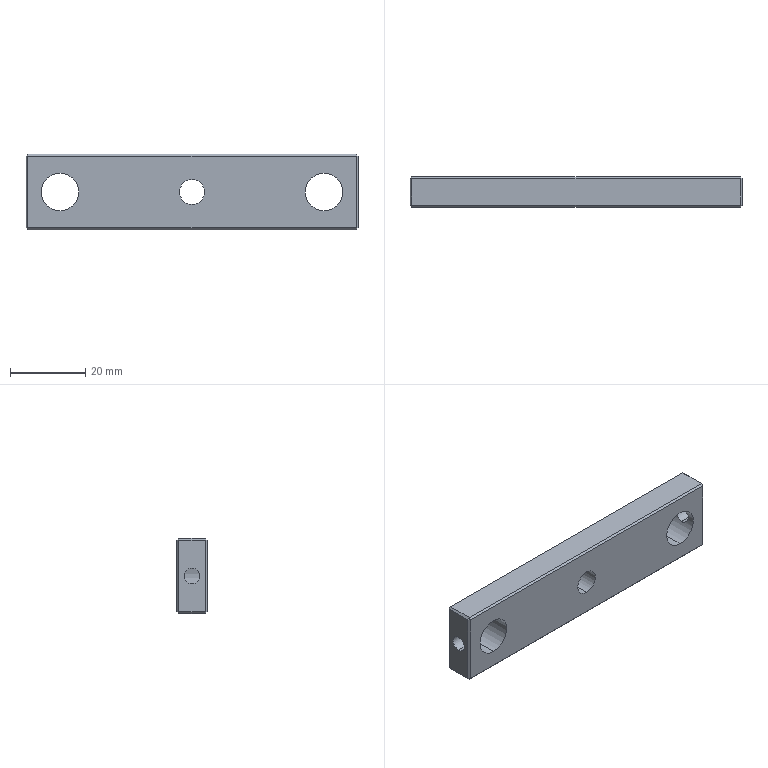Part | SolidWorks | features HoleWzd 3, Chamfer 1, Extrusion 1, ICE 1 | 1 solid | 39 faces | box 88 x 8 x 20 mm | volume 12196 mm3 | plane 27 | cylinder 12 | commonest cylinder face diameters 4.2 x4 10 x4 6.6 x2 11 x2
STEP:
#1=CARTESIAN_POINT('',(39.538,4.,2.1));
#2=VERTEX_POINT('',#1);
#3=CARTESIAN_POINT('',(39.538,4.,-2.1));
#4=VERTEX_POINT('',#3);
#5=CARTESIAN_POINT('',(39.538,4.,2.1));
#6=CARTESIAN_POINT('',(39.538,3.862,2.1));
#7=CARTESIAN_POINT('',(39.544,3.721,2.086));
#8=CARTESIAN_POINT('',(39.569,3.449,2.031));
#9=CARTESIAN_POINT('',(39.587,3.318,1.991));
#10=CARTESIAN_POINT('',(39.654,2.937,1.832));
#11=CARTESIAN_POINT('',(39.714,2.708,1.678));
#12=CARTESIAN_POINT('',(39.805,2.418,1.388));
#13=CARTESIAN_POINT('',(39.834,2.332,1.283));
#14=CARTESIAN_POINT('',(39.888,2.181,1.058));
#15=CARTESIAN_POINT('',(39.913,2.115,0.9354));
#16=CARTESIAN_POINT('',(39.955,2.009,0.682));
#17=CARTESIAN_POINT('',(39.971,1.969,0.551));
#18=CARTESIAN_POINT('',(39.994,1.914,0.2796));
#19=CARTESIAN_POINT('',(40.,1.9,0.1388));
#20=CARTESIAN_POINT('',(40.,1.9,-0.2766));
#21=CARTESIAN_POINT('',(39.976,1.956,-0.5557));
#22=CARTESIAN_POINT('',(39.913,2.115,-0.9355));
#23=CARTESIAN_POINT('',(39.888,2.181,-1.058));
#24=CARTESIAN_POINT('',(39.834,2.333,-1.284));
#25=CARTESIAN_POINT('',(39.804,2.419,-1.389));
#26=CARTESIAN_POINT('',(39.744,2.612,-1.582));
#27=CARTESIAN_POINT('',(39.714,2.718,-1.669));
#28=CARTESIAN_POINT('',(39.658,2.943,-1.82));
#29=CARTESIAN_POINT('',(39.632,3.063,-1.885));
#30=CARTESIAN_POINT('',(39.587,3.319,-1.991));
#31=CARTESIAN_POINT('',(39.569,3.45,-2.031));
#32=CARTESIAN_POINT('',(39.544,3.72,-2.086));
#33=CARTESIAN_POINT('',(39.538,3.86,-2.1));
#34=CARTESIAN_POINT('',(39.538,4.,-2.1));
#35=B_SPLINE_CURVE_WITH_KNOTS('',3,(#5,#6,#7,#8,#9,#10,#11,#12,#13,#14,#15,#16,#17,#18,#19,#20,#21,#22,#23,#24,#25,#26,#27,#28,#29,#30,#31,#32,#33,#34),.UNSPECIFIED.,.F.,.F.,(4,2,2,2,2,2,2,2,2,2,2,2,2,2,4),(0.006643,0.007058,0.007473,0.008303,0.008717,0.009132,0.009547,0.009962,0.01079,0.01121,0.01162,0.01204,0.01245,0.01287,0.01328),.UNSPECIFIED.);
#36=EDGE_CURVE('',#2,#4,#35,.T.);
#37=ORIENTED_EDGE('',*,*,#36,.F.);
#38=CARTESIAN_POINT('',(44.,4.,2.1));
#39=VERTEX_POINT('',#38);
#40=CARTESIAN_POINT('',(44.,4.,2.1));
#41=DIRECTION('',(1.,0.,0.));
#42=VECTOR('',#41,1000.);
#43=LINE('',#40,#42);
#44=EDGE_CURVE('',#2,#39,#43,.T.);
#45=ORIENTED_EDGE('',*,*,#44,.T.);
#46=CARTESIAN_POINT('',(44.,4.,-2.1));
#47=VERTEX_POINT('',#46);
#48=CARTESIAN_POINT('',(44.,4.,0.));
#49=DIRECTION('',(1.,0.,0.));
#50=DIRECTION('',(0.,0.,-1.));
#51=AXIS2_PLACEMENT_3D('',#48,#49,#50);
#52=CIRCLE('',#51,2.1);
#53=EDGE_CURVE('',#39,#47,#52,.T.);
#54=ORIENTED_EDGE('',*,*,#53,.T.);
#55=CARTESIAN_POINT('',(44.,4.,-2.1));
#56=DIRECTION('',(1.,0.,0.));
#57=VECTOR('',#56,1000.);
#58=LINE('',#55,#57);
#59=EDGE_CURVE('',#4,#47,#58,.T.);
#60=ORIENTED_EDGE('',*,*,#59,.F.);
#61=EDGE_LOOP('',(#37,#45,#54,#60));
#62=FACE_OUTER_BOUND('',#61,.T.);
#63=CARTESIAN_POINT('',(44.,4.,0.));
#64=DIRECTION('',(1.,0.,0.));
#65=DIRECTION('',(0.,0.,-1.));
#66=AXIS2_PLACEMENT_3D('',#63,#64,#65);
#67=CYLINDRICAL_SURFACE('',#66,2.1);
#68=ADVANCED_FACE('',(#62),#67,.F.);
#69=CARTESIAN_POINT('',(-39.538,4.,-2.1));
#70=VERTEX_POINT('',#69);
#71=CARTESIAN_POINT('',(-39.538,4.,2.1));
#72=VERTEX_POINT('',#71);
#73=CARTESIAN_POINT('',(-39.538,4.,-2.1));
#74=CARTESIAN_POINT('',(-39.538,3.862,-2.1));
#75=CARTESIAN_POINT('',(-39.544,3.721,-2.086));
#76=CARTESIAN_POINT('',(-39.569,3.449,-2.031));
#77=CARTESIAN_POINT('',(-39.587,3.318,-1.991));
#78=CARTESIAN_POINT('',(-39.654,2.937,-1.832));
#79=CARTESIAN_POINT('',(-39.714,2.708,-1.678));
#80=CARTESIAN_POINT('',(-39.805,2.418,-1.388));
#81=CARTESIAN_POINT('',(-39.834,2.332,-1.283));
#82=CARTESIAN_POINT('',(-39.888,2.181,-1.058));
#83=CARTESIAN_POINT('',(-39.913,2.115,-0.9354));
#84=CARTESIAN_POINT('',(-39.955,2.009,-0.682));
#85=CARTESIAN_POINT('',(-39.971,1.969,-0.551));
#86=CARTESIAN_POINT('',(-39.994,1.914,-0.2796));
#87=CARTESIAN_POINT('',(-40.,1.9,-0.1388));
#88=CARTESIAN_POINT('',(-40.,1.9,0.2766));
#89=CARTESIAN_POINT('',(-39.976,1.956,0.5557));
#90=CARTESIAN_POINT('',(-39.913,2.115,0.9355));
#91=CARTESIAN_POINT('',(-39.888,2.181,1.058));
#92=CARTESIAN_POINT('',(-39.834,2.333,1.284));
#93=CARTESIAN_POINT('',(-39.804,2.419,1.389));
#94=CARTESIAN_POINT('',(-39.744,2.612,1.582));
#95=CARTESIAN_POINT('',(-39.714,2.718,1.669));
#96=CARTESIAN_POINT('',(-39.658,2.943,1.82));
#97=CARTESIAN_POINT('',(-39.632,3.063,1.885));
#98=CARTESIAN_POINT('',(-39.587,3.319,1.991));
#99=CARTESIAN_POINT('',(-39.569,3.45,2.031));
#100=CARTESIAN_POINT('',(-39.544,3.72,2.086));
#101=CARTESIAN_POINT('',(-39.538,3.86,2.1));
#102=CARTESIAN_POINT('',(-39.538,4.,2.1));
#103=B_SPLINE_CURVE_WITH_KNOTS('',3,(#73,#74,#75,#76,#77,#78,#79,#80,#81,#82,#83,#84,#85,#86,#87,#88,#89,#90,#91,#92,#93,#94,#95,#96,#97,#98,#99,#100,#101,#102),.UNSPECIFIED.,.F.,.F.,(4,2,2,2,2,2,2,2,2,2,2,2,2,2,4),(0.006643,0.007058,0.007473,0.008303,0.008717,0.009132,0.009547,0.009962,0.01079,0.01121,0.01162,0.01204,0.01245,0.01287,0.01328),.UNSPECIFIED.);
#104=EDGE_CURVE('',#70,#72,#103,.T.);
#105=ORIENTED_EDGE('',*,*,#104,.F.);
#106=CARTESIAN_POINT('',(-44.,4.,-2.1));
#107=VERTEX_POINT('',#106);
#108=CARTESIAN_POINT('',(-44.,4.,-2.1));
#109=DIRECTION('',(-1.,0.,0.));
#110=VECTOR('',#109,1000.);
#111=LINE('',#108,#110);
#112=EDGE_CURVE('',#70,#107,#111,.T.);
#113=ORIENTED_EDGE('',*,*,#112,.T.);
#114=CARTESIAN_POINT('',(-44.,4.,2.1));
#115=VERTEX_POINT('',#114);
#116=CARTESIAN_POINT('',(-44.,4.,0.));
#117=DIRECTION('',(-1.,0.,0.));
#118=DIRECTION('',(0.,0.,1.));
#119=AXIS2_PLACEMENT_3D('',#116,#117,#118);
#120=CIRCLE('',#119,2.1);
#121=EDGE_CURVE('',#107,#115,#120,.T.);
#122=ORIENTED_EDGE('',*,*,#121,.T.);
#123=CARTESIAN_POINT('',(-44.,4.,2.1));
#124=DIRECTION('',(-1.,0.,0.));
#125=VECTOR('',#124,1000.);
#126=LINE('',#123,#125);
#127=EDGE_CURVE('',#72,#115,#126,.T.);
#128=ORIENTED_EDGE('',*,*,#127,.F.);
#129=EDGE_LOOP('',(#105,#113,#122,#128));
#130=FACE_OUTER_BOUND('',#129,.T.);
#131=CARTESIAN_POINT('',(-44.,4.,0.));
#132=DIRECTION('',(-1.,0.,0.));
#133=DIRECTION('',(0.,0.,1.));
#134=AXIS2_PLACEMENT_3D('',#131,#132,#133);
#135=CYLINDRICAL_SURFACE('',#134,2.1);
#136=ADVANCED_FACE('',(#130),#135,.F.);
#137=CARTESIAN_POINT('',(0.,5.,-5.5));
#138=VERTEX_POINT('',#137);
#139=CARTESIAN_POINT('',(0.,5.,5.5));
#140=VERTEX_POINT('',#139);
#141=CARTESIAN_POINT('',(0.,5.,0.));
#142=DIRECTION('',(0.,1.,0.));
#143=DIRECTION('',(0.,0.,1.));
#144=AXIS2_PLACEMENT_3D('',#141,#142,#143);
#145=CIRCLE('',#144,5.5);
#146=EDGE_CURVE('',#138,#140,#145,.T.);
#147=ORIENTED_EDGE('',*,*,#146,.F.);
#148=CARTESIAN_POINT('',(0.,8.,-5.5));
#149=VERTEX_POINT('',#148);
#150=CARTESIAN_POINT('',(0.,8.,-5.5));
#151=DIRECTION('',(0.,1.,0.));
#152=VECTOR('',#151,1000.);
#153=LINE('',#150,#152);
#154=EDGE_CURVE('',#138,#149,#153,.T.);
#155=ORIENTED_EDGE('',*,*,#154,.T.);
#156=CARTESIAN_POINT('',(0.,8.,5.5));
#157=VERTEX_POINT('',#156);
#158=CARTESIAN_POINT('',(0.,8.,0.));
#159=DIRECTION('',(0.,1.,0.));
#160=DIRECTION('',(0.,0.,1.));
#161=AXIS2_PLACEMENT_3D('',#158,#159,#160);
#162=CIRCLE('',#161,5.5);
#163=EDGE_CURVE('',#149,#157,#162,.T.);
#164=ORIENTED_EDGE('',*,*,#163,.T.);
#165=CARTESIAN_POINT('',(0.,8.,5.5));
#166=DIRECTION('',(0.,1.,0.));
#167=VECTOR('',#166,1000.);
#168=LINE('',#165,#167);
#169=EDGE_CURVE('',#140,#157,#168,.T.);
#170=ORIENTED_EDGE('',*,*,#169,.F.);
#171=EDGE_LOOP('',(#147,#155,#164,#170));
#172=FACE_OUTER_BOUND('',#171,.T.);
#173=CARTESIAN_POINT('',(0.,8.,0.));
#174=DIRECTION('',(0.,1.,0.));
#175=DIRECTION('',(0.,0.,1.));
#176=AXIS2_PLACEMENT_3D('',#173,#174,#175);
#177=CYLINDRICAL_SURFACE('',#176,5.5);
#178=ADVANCED_FACE('',(#172),#177,.F.);
#179=CARTESIAN_POINT('',(0.,0.,-3.3));
#180=VERTEX_POINT('',#179);
#181=CARTESIAN_POINT('',(0.,0.,3.3));
#182=VERTEX_POINT('',#181);
#183=CARTESIAN_POINT('',(0.,0.,0.));
#184=DIRECTION('',(0.,1.,0.));
#185=DIRECTION('',(0.,0.,1.));
#186=AXIS2_PLACEMENT_3D('',#183,#184,#185);
#187=CIRCLE('',#186,3.3);
#188=EDGE_CURVE('',#180,#182,#187,.T.);
#189=ORIENTED_EDGE('',*,*,#188,.F.);
#190=CARTESIAN_POINT('',(0.,5.,-3.3));
#191=VERTEX_POINT('',#190);
#192=CARTESIAN_POINT('',(0.,8.,-3.3));
#193=DIRECTION('',(0.,1.,0.));
#194=VECTOR('',#193,1000.);
#195=LINE('',#192,#194);
#196=EDGE_CURVE('',#180,#191,#195,.T.);
#197=ORIENTED_EDGE('',*,*,#196,.T.);
#198=CARTESIAN_POINT('',(0.,5.,3.3));
#199=VERTEX_POINT('',#198);
#200=CARTESIAN_POINT('',(0.,5.,0.));
#201=DIRECTION('',(0.,1.,0.));
#202=DIRECTION('',(0.,0.,1.));
#203=AXIS2_PLACEMENT_3D('',#200,#201,#202);
#204=CIRCLE('',#203,3.3);
#205=EDGE_CURVE('',#191,#199,#204,.T.);
#206=ORIENTED_EDGE('',*,*,#205,.T.);
#207=CARTESIAN_POINT('',(0.,8.,3.3));
#208=DIRECTION('',(0.,1.,0.));
#209=VECTOR('',#208,1000.);
#210=LINE('',#207,#209);
#211=EDGE_CURVE('',#182,#199,#210,.T.);
#212=ORIENTED_EDGE('',*,*,#211,.F.);
#213=EDGE_LOOP('',(#189,#197,#206,#212));
#214=FACE_OUTER_BOUND('',#213,.T.);
#215=CARTESIAN_POINT('',(0.,8.,0.));
#216=DIRECTION('',(0.,1.,0.));
#217=DIRECTION('',(0.,0.,1.));
#218=AXIS2_PLACEMENT_3D('',#215,#216,#217);
#219=CYLINDRICAL_SURFACE('',#218,3.3);
#220=ADVANCED_FACE('',(#214),#219,.F.);
#221=CARTESIAN_POINT('',(35.,8.,5.));
#222=VERTEX_POINT('',#221);
#223=CARTESIAN_POINT('',(35.,8.,-5.));
#224=VERTEX_POINT('',#223);
#225=CARTESIAN_POINT('',(35.,8.,0.));
#226=DIRECTION('',(0.,-1.,0.));
#227=DIRECTION('',(0.,0.,-1.));
#228=AXIS2_PLACEMENT_3D('',#225,#226,#227);
#229=CIRCLE('',#228,5.);
#230=EDGE_CURVE('',#222,#224,#229,.T.);
#231=ORIENTED_EDGE('',*,*,#230,.F.);
#232=CARTESIAN_POINT('',(35.,0.,5.));
#233=VERTEX_POINT('',#232);
#234=CARTESIAN_POINT('',(35.,8.,5.));
#235=DIRECTION('',(0.,-1.,0.));
#236=VECTOR('',#235,1000.);
#237=LINE('',#234,#236);
#238=EDGE_CURVE('',#222,#233,#237,.T.);
#239=ORIENTED_EDGE('',*,*,#238,.T.);
#240=CARTESIAN_POINT('',(35.,0.,-5.));
#241=VERTEX_POINT('',#240);
#242=CARTESIAN_POINT('',(35.,0.,0.));
#243=DIRECTION('',(0.,-1.,0.));
#244=DIRECTION('',(0.,0.,-1.));
#245=AXIS2_PLACEMENT_3D('',#242,#243,#244);
#246=CIRCLE('',#245,5.);
#247=EDGE_CURVE('',#233,#241,#246,.T.);
#248=ORIENTED_EDGE('',*,*,#247,.T.);
#249=CARTESIAN_POINT('',(35.,8.,-5.));
#250=DIRECTION('',(0.,-1.,0.));
#251=VECTOR('',#250,1000.);
#252=LINE('',#249,#251);
#253=EDGE_CURVE('',#224,#241,#252,.T.);
#254=ORIENTED_EDGE('',*,*,#253,.F.);
#255=EDGE_LOOP('',(#231,#239,#248,#254));
#256=FACE_OUTER_BOUND('',#255,.T.);
#257=CARTESIAN_POINT('',(35.,8.,0.));
#258=DIRECTION('',(0.,-1.,0.));
#259=DIRECTION('',(0.,0.,-1.));
#260=AXIS2_PLACEMENT_3D('',#257,#258,#259);
#261=CYLINDRICAL_SURFACE('',#260,5.);
#262=ADVANCED_FACE('',(#256),#261,.F.);
#263=CARTESIAN_POINT('',(-39.538,4.,2.1));
#264=CARTESIAN_POINT('',(-39.538,4.141,2.1));
#265=CARTESIAN_POINT('',(-39.544,4.278,2.086));
#266=CARTESIAN_POINT('',(-39.569,4.549,2.032));
#267=CARTESIAN_POINT('',(-39.587,4.683,1.991));
#268=CARTESIAN_POINT('',(-39.632,4.936,1.885));
#269=CARTESIAN_POINT('',(-39.658,5.056,1.82));
#270=CARTESIAN_POINT('',(-39.714,5.283,1.668));
#271=CARTESIAN_POINT('',(-39.745,5.389,1.581));
#272=CARTESIAN_POINT('',(-39.834,5.676,1.294));
#273=CARTESIAN_POINT('',(-39.893,5.832,1.062));
#274=CARTESIAN_POINT('',(-39.955,5.99,0.6836));
#275=CARTESIAN_POINT('',(-39.972,6.032,0.5495));
#276=CARTESIAN_POINT('',(-39.994,6.086,0.2775));
#277=CARTESIAN_POINT('',(-40.,6.1,0.1401));
#278=CARTESIAN_POINT('',(-40.,6.1,-0.1378));
#279=CARTESIAN_POINT('',(-39.994,6.086,-0.2786));
#280=CARTESIAN_POINT('',(-39.972,6.032,-0.5496));
#281=CARTESIAN_POINT('',(-39.955,5.991,-0.6819));
#282=CARTESIAN_POINT('',(-39.913,5.884,-0.9378));
#283=CARTESIAN_POINT('',(-39.888,5.819,-1.058));
#284=CARTESIAN_POINT('',(-39.834,5.667,-1.284));
#285=CARTESIAN_POINT('',(-39.804,5.579,-1.391));
#286=CARTESIAN_POINT('',(-39.744,5.387,-1.582));
#287=CARTESIAN_POINT('',(-39.714,5.283,-1.668));
#288=CARTESIAN_POINT('',(-39.658,5.056,-1.82));
#289=CARTESIAN_POINT('',(-39.631,4.934,-1.886));
#290=CARTESIAN_POINT('',(-39.565,4.556,-2.043));
#291=CARTESIAN_POINT('',(-39.538,4.277,-2.1));
#292=CARTESIAN_POINT('',(-39.538,4.,-2.1));
#293=B_SPLINE_CURVE_WITH_KNOTS('',3,(#263,#264,#265,#266,#267,#268,#269,#270,#271,#272,#273,#274,#275,#276,#277,#278,#279,#280,#281,#282,#283,#284,#285,#286,#287,#288,#289,#290,#291,#292),.UNSPECIFIED.,.F.,.F.,(4,2,2,2,2,2,2,2,2,2,2,2,2,2,4),(0.,0.0004152,0.0008304,0.001246,0.001661,0.002491,0.002906,0.003322,0.003737,0.004152,0.004567,0.004982,0.005398,0.005813,0.006643),.UNSPECIFIED.);
#294=EDGE_CURVE('',#72,#70,#293,.T.);
#295=ORIENTED_EDGE('',*,*,#294,.T.);
#296=ORIENTED_EDGE('',*,*,#104,.T.);
#297=EDGE_LOOP('',(#295,#296));
#298=FACE_BOUND('',#297,.T.);
#299=CARTESIAN_POINT('',(-35.,8.,5.));
#300=VERTEX_POINT('',#299);
#301=CARTESIAN_POINT('',(-35.,8.,-5.));
#302=VERTEX_POINT('',#301);
#303=CARTESIAN_POINT('',(-35.,8.,0.));
#304=DIRECTION('',(0.,-1.,0.));
#305=DIRECTION('',(0.,0.,-1.));
#306=AXIS2_PLACEMENT_3D('',#303,#304,#305);
#307=CIRCLE('',#306,5.);
#308=EDGE_CURVE('',#300,#302,#307,.T.);
#309=ORIENTED_EDGE('',*,*,#308,.F.);
#310=CARTESIAN_POINT('',(-35.,0.,5.));
#311=VERTEX_POINT('',#310);
#312=CARTESIAN_POINT('',(-35.,8.,5.));
#313=DIRECTION('',(0.,-1.,0.));
#314=VECTOR('',#313,1000.);
#315=LINE('',#312,#314);
#316=EDGE_CURVE('',#300,#311,#315,.T.);
#317=ORIENTED_EDGE('',*,*,#316,.T.);
#318=CARTESIAN_POINT('',(-35.,0.,-5.));
#319=VERTEX_POINT('',#318);
#320=CARTESIAN_POINT('',(-35.,0.,0.));
#321=DIRECTION('',(0.,-1.,0.));
#322=DIRECTION('',(0.,0.,-1.));
#323=AXIS2_PLACEMENT_3D('',#320,#321,#322);
#324=CIRCLE('',#323,5.);
#325=EDGE_CURVE('',#311,#319,#324,.T.);
#326=ORIENTED_EDGE('',*,*,#325,.T.);
#327=CARTESIAN_POINT('',(-35.,8.,-5.));
#328=DIRECTION('',(0.,-1.,0.));
#329=VECTOR('',#328,1000.);
#330=LINE('',#327,#329);
#331=EDGE_CURVE('',#302,#319,#330,.T.);
#332=ORIENTED_EDGE('',*,*,#331,.F.);
#333=EDGE_LOOP('',(#309,#317,#326,#332));
#334=FACE_OUTER_BOUND('',#333,.T.);
#335=CARTESIAN_POINT('',(-35.,8.,0.));
#336=DIRECTION('',(0.,-1.,0.));
#337=DIRECTION('',(0.,0.,-1.));
#338=AXIS2_PLACEMENT_3D('',#335,#336,#337);
#339=CYLINDRICAL_SURFACE('',#338,5.);
#340=ADVANCED_FACE('',(#298,#334),#339,.F.);
#341=CARTESIAN_POINT('',(44.,4.,0.));
#342=DIRECTION('',(1.,0.,0.));
#343=DIRECTION('',(0.,0.,-1.));
#344=AXIS2_PLACEMENT_3D('',#341,#342,#343);
#345=CIRCLE('',#344,2.1);
#346=EDGE_CURVE('',#47,#39,#345,.T.);
#347=ORIENTED_EDGE('',*,*,#346,.F.);
#348=ORIENTED_EDGE('',*,*,#53,.F.);
#349=EDGE_LOOP('',(#347,#348));
#350=FACE_BOUND('',#349,.T.);
#351=CARTESIAN_POINT('',(44.,0.5,9.5));
#352=VERTEX_POINT('',#351);
#353=CARTESIAN_POINT('',(44.,0.5,-9.5));
#354=VERTEX_POINT('',#353);
#355=CARTESIAN_POINT('',(44.,0.5,-10.));
#356=DIRECTION('',(0.,0.,-1.));
#357=VECTOR('',#356,1000.);
#358=LINE('',#355,#357);
#359=EDGE_CURVE('',#352,#354,#358,.T.);
#360=ORIENTED_EDGE('',*,*,#359,.T.);
#361=CARTESIAN_POINT('',(44.,7.5,-9.5));
#362=VERTEX_POINT('',#361);
#363=CARTESIAN_POINT('',(44.,8.,-9.5));
#364=DIRECTION('',(0.,1.,0.));
#365=VECTOR('',#364,1000.);
#366=LINE('',#363,#365);
#367=EDGE_CURVE('',#354,#362,#366,.T.);
#368=ORIENTED_EDGE('',*,*,#367,.T.);
#369=CARTESIAN_POINT('',(44.,7.5,9.5));
#370=VERTEX_POINT('',#369);
#371=CARTESIAN_POINT('',(44.,7.5,10.));
#372=DIRECTION('',(0.,0.,1.));
#373=VECTOR('',#372,1000.);
#374=LINE('',#371,#373);
#375=EDGE_CURVE('',#362,#370,#374,.T.);
#376=ORIENTED_EDGE('',*,*,#375,.T.);
#377=CARTESIAN_POINT('',(44.,8.,9.5));
#378=DIRECTION('',(0.,-1.,0.));
#379=VECTOR('',#378,1000.);
#380=LINE('',#377,#379);
#381=EDGE_CURVE('',#370,#352,#380,.T.);
#382=ORIENTED_EDGE('',*,*,#381,.T.);
#383=EDGE_LOOP('',(#360,#368,#376,#382));
#384=FACE_OUTER_BOUND('',#383,.T.);
#385=CARTESIAN_POINT('',(44.,8.,-10.));
#386=DIRECTION('',(-1.,0.,0.));
#387=DIRECTION('',(0.,0.,1.));
#388=AXIS2_PLACEMENT_3D('',#385,#386,#387);
#389=PLANE('',#388);
#390=ADVANCED_FACE('',(#350,#384),#389,.F.);
#391=CARTESIAN_POINT('',(43.5,7.5,-10.));
#392=VERTEX_POINT('',#391);
#393=CARTESIAN_POINT('',(43.5,0.5,-10.));
#394=VERTEX_POINT('',#393);
#395=CARTESIAN_POINT('',(43.5,8.,-10.));
#396=DIRECTION('',(0.,-1.,0.));
#397=VECTOR('',#396,1000.);
#398=LINE('',#395,#397);
#399=EDGE_CURVE('',#392,#394,#398,.T.);
#400=ORIENTED_EDGE('',*,*,#399,.T.);
#401=CARTESIAN_POINT('',(-43.5,0.5,-10.));
#402=VERTEX_POINT('',#401);
#403=CARTESIAN_POINT('',(-44.,0.5,-10.));
#404=DIRECTION('',(-1.,0.,0.));
#405=VECTOR('',#404,1000.);
#406=LINE('',#403,#405);
#407=EDGE_CURVE('',#394,#402,#406,.T.);
#408=ORIENTED_EDGE('',*,*,#407,.T.);
#409=CARTESIAN_POINT('',(-43.5,7.5,-10.));
#410=VERTEX_POINT('',#409);
#411=CARTESIAN_POINT('',(-43.5,8.,-10.));
#412=DIRECTION('',(0.,1.,0.));
#413=VECTOR('',#412,1000.);
#414=LINE('',#411,#413);
#415=EDGE_CURVE('',#402,#410,#414,.T.);
#416=ORIENTED_EDGE('',*,*,#415,.T.);
#417=CARTESIAN_POINT('',(44.,7.5,-10.));
#418=DIRECTION('',(1.,0.,0.));
#419=VECTOR('',#418,1000.);
#420=LINE('',#417,#419);
#421=EDGE_CURVE('',#410,#392,#420,.T.);
#422=ORIENTED_EDGE('',*,*,#421,.T.);
#423=EDGE_LOOP('',(#400,#408,#416,#422));
#424=FACE_OUTER_BOUND('',#423,.T.);
#425=CARTESIAN_POINT('',(-44.,8.,-10.));
#426=DIRECTION('',(0.,0.,1.));
#427=DIRECTION('',(1.,0.,0.));
#428=AXIS2_PLACEMENT_3D('',#425,#426,#427);
#429=PLANE('',#428);
#430=ADVANCED_FACE('',(#424),#429,.F.);
#431=CARTESIAN_POINT('',(-44.,4.,0.));
#432=DIRECTION('',(-1.,0.,0.));
#433=DIRECTION('',(0.,0.,1.));
#434=AXIS2_PLACEMENT_3D('',#431,#432,#433);
#435=CIRCLE('',#434,2.1);
#436=EDGE_CURVE('',#115,#107,#435,.T.);
#437=ORIENTED_EDGE('',*,*,#436,.F.);
#438=ORIENTED_EDGE('',*,*,#121,.F.);
#439=EDGE_LOOP('',(#437,#438));
#440=FACE_BOUND('',#439,.T.);
#441=CARTESIAN_POINT('',(-44.,7.5,-9.5));
#442=VERTEX_POINT('',#441);
#443=CARTESIAN_POINT('',(-44.,0.5,-9.5));
#444=VERTEX_POINT('',#443);
#445=CARTESIAN_POINT('',(-44.,8.,-9.5));
#446=DIRECTION('',(0.,-1.,0.));
#447=VECTOR('',#446,1000.);
#448=LINE('',#445,#447);
#449=EDGE_CURVE('',#442,#444,#448,.T.);
#450=ORIENTED_EDGE('',*,*,#449,.T.);
#451=CARTESIAN_POINT('',(-44.,0.5,9.5));
#452=VERTEX_POINT('',#451);
#453=CARTESIAN_POINT('',(-44.,0.5,-10.));
#454=DIRECTION('',(0.,0.,1.));
#455=VECTOR('',#454,1000.);
#456=LINE('',#453,#455);
#457=EDGE_CURVE('',#444,#452,#456,.T.);
#458=ORIENTED_EDGE('',*,*,#457,.T.);
#459=CARTESIAN_POINT('',(-44.,7.5,9.5));
#460=VERTEX_POINT('',#459);
#461=CARTESIAN_POINT('',(-44.,8.,9.5));
#462=DIRECTION('',(0.,1.,0.));
#463=VECTOR('',#462,1000.);
#464=LINE('',#461,#463);
#465=EDGE_CURVE('',#452,#460,#464,.T.);
#466=ORIENTED_EDGE('',*,*,#465,.T.);
#467=CARTESIAN_POINT('',(-44.,7.5,-10.));
#468=DIRECTION('',(0.,0.,-1.));
#469=VECTOR('',#468,1000.);
#470=LINE('',#467,#469);
#471=EDGE_CURVE('',#460,#442,#470,.T.);
#472=ORIENTED_EDGE('',*,*,#471,.T.);
#473=EDGE_LOOP('',(#450,#458,#466,#472));
#474=FACE_OUTER_BOUND('',#473,.T.);
#475=CARTESIAN_POINT('',(-44.,8.,-10.));
#476=DIRECTION('',(1.,0.,0.));
#477=DIRECTION('',(0.,0.,-1.));
#478=AXIS2_PLACEMENT_3D('',#475,#476,#477);
#479=PLANE('',#478);
#480=ADVANCED_FACE('',(#440,#474),#479,.F.);
#481=CARTESIAN_POINT('',(43.5,7.5,10.));
#482=VERTEX_POINT('',#481);
#483=CARTESIAN_POINT('',(-43.5,7.5,10.));
#484=VERTEX_POINT('',#483);
#485=CARTESIAN_POINT('',(-44.,7.5,10.));
#486=DIRECTION('',(-1.,0.,0.));
#487=VECTOR('',#486,1000.);
#488=LINE('',#485,#487);
#489=EDGE_CURVE('',#482,#484,#488,.T.);
#490=ORIENTED_EDGE('',*,*,#489,.T.);
#491=CARTESIAN_POINT('',(-43.5,0.5,10.));
#492=VERTEX_POINT('',#491);
#493=CARTESIAN_POINT('',(-43.5,8.,10.));
#494=DIRECTION('',(0.,-1.,0.));
#495=VECTOR('',#494,1000.);
#496=LINE('',#493,#495);
#497=EDGE_CURVE('',#484,#492,#496,.T.);
#498=ORIENTED_EDGE('',*,*,#497,.T.);
#499=CARTESIAN_POINT('',(43.5,0.5,10.));
#500=VERTEX_POINT('',#499);
#501=CARTESIAN_POINT('',(-44.,0.5,10.));
#502=DIRECTION('',(1.,0.,0.));
#503=VECTOR('',#502,1000.);
#504=LINE('',#501,#503);
#505=EDGE_CURVE('',#492,#500,#504,.T.);
#506=ORIENTED_EDGE('',*,*,#505,.T.);
#507=CARTESIAN_POINT('',(43.5,8.,10.));
#508=DIRECTION('',(0.,1.,0.));
#509=VECTOR('',#508,1000.);
#510=LINE('',#507,#509);
#511=EDGE_CURVE('',#500,#482,#510,.T.);
#512=ORIENTED_EDGE('',*,*,#511,.T.);
#513=EDGE_LOOP('',(#490,#498,#506,#512));
#514=FACE_OUTER_BOUND('',#513,.T.);
#515=CARTESIAN_POINT('',(-44.,8.,10.));
#516=DIRECTION('',(0.,0.,-1.));
#517=DIRECTION('',(-1.,0.,0.));
#518=AXIS2_PLACEMENT_3D('',#515,#516,#517);
#519=PLANE('',#518);
#520=ADVANCED_FACE('',(#514),#519,.F.);
#521=CARTESIAN_POINT('',(0.,8.,0.));
#522=DIRECTION('',(0.,1.,0.));
#523=DIRECTION('',(0.,0.,1.));
#524=AXIS2_PLACEMENT_3D('',#521,#522,#523);
#525=CIRCLE('',#524,5.5);
#526=EDGE_CURVE('',#157,#149,#525,.T.);
#527=ORIENTED_EDGE('',*,*,#526,.F.);
#528=ORIENTED_EDGE('',*,*,#163,.F.);
#529=EDGE_LOOP('',(#527,#528));
#530=FACE_BOUND('',#529,.T.);
#531=CARTESIAN_POINT('',(35.,8.,0.));
#532=DIRECTION('',(0.,-1.,0.));
#533=DIRECTION('',(0.,0.,-1.));
#534=AXIS2_PLACEMENT_3D('',#531,#532,#533);
#535=CIRCLE('',#534,5.);
#536=EDGE_CURVE('',#224,#222,#535,.T.);
#537=ORIENTED_EDGE('',*,*,#536,.T.);
#538=ORIENTED_EDGE('',*,*,#230,.T.);
#539=EDGE_LOOP('',(#537,#538));
#540=FACE_BOUND('',#539,.T.);
#541=CARTESIAN_POINT('',(-35.,8.,0.));
#542=DIRECTION('',(0.,-1.,0.));
#543=DIRECTION('',(0.,0.,-1.));
#544=AXIS2_PLACEMENT_3D('',#541,#542,#543);
#545=CIRCLE('',#544,5.);
#546=EDGE_CURVE('',#302,#300,#545,.T.);
#547=ORIENTED_EDGE('',*,*,#546,.T.);
#548=ORIENTED_EDGE('',*,*,#308,.T.);
#549=EDGE_LOOP('',(#547,#548));
#550=FACE_BOUND('',#549,.T.);
#551=CARTESIAN_POINT('',(-43.5,8.,-9.5));
#552=VERTEX_POINT('',#551);
#553=CARTESIAN_POINT('',(-43.5,8.,9.5));
#554=VERTEX_POINT('',#553);
#555=CARTESIAN_POINT('',(-43.5,8.,10.));
#556=DIRECTION('',(0.,0.,1.));
#557=VECTOR('',#556,1000.);
#558=LINE('',#555,#557);
#559=EDGE_CURVE('',#552,#554,#558,.T.);
#560=ORIENTED_EDGE('',*,*,#559,.T.);
#561=CARTESIAN_POINT('',(43.5,8.,9.5));
#562=VERTEX_POINT('',#561);
#563=CARTESIAN_POINT('',(44.,8.,9.5));
#564=DIRECTION('',(1.,0.,0.));
#565=VECTOR('',#564,1000.);
#566=LINE('',#563,#565);
#567=EDGE_CURVE('',#554,#562,#566,.T.);
#568=ORIENTED_EDGE('',*,*,#567,.T.);
#569=CARTESIAN_POINT('',(43.5,8.,-9.5));
#570=VERTEX_POINT('',#569);
#571=CARTESIAN_POINT('',(43.5,8.,-10.));
#572=DIRECTION('',(0.,0.,-1.));
#573=VECTOR('',#572,1000.);
#574=LINE('',#571,#573);
#575=EDGE_CURVE('',#562,#570,#574,.T.);
#576=ORIENTED_EDGE('',*,*,#575,.T.);
#577=CARTESIAN_POINT('',(-44.,8.,-9.5));
#578=DIRECTION('',(-1.,0.,0.));
#579=VECTOR('',#578,1000.);
#580=LINE('',#577,#579);
#581=EDGE_CURVE('',#570,#552,#580,.T.);
#582=ORIENTED_EDGE('',*,*,#581,.T.);
#583=EDGE_LOOP('',(#560,#568,#576,#582));
#584=FACE_OUTER_BOUND('',#583,.T.);
#585=CARTESIAN_POINT('',(0.,8.,0.));
#586=DIRECTION('',(0.,1.,0.));
#587=DIRECTION('',(0.,0.,1.));
#588=AXIS2_PLACEMENT_3D('',#585,#586,#587);
#589=PLANE('',#588);
#590=ADVANCED_FACE('',(#530,#540,#550,#584),#589,.T.);
#591=CARTESIAN_POINT('',(0.,0.,0.));
#592=DIRECTION('',(0.,1.,0.));
#593=DIRECTION('',(0.,0.,1.));
#594=AXIS2_PLACEMENT_3D('',#591,#592,#593);
#595=CIRCLE('',#594,3.3);
#596=EDGE_CURVE('',#182,#180,#595,.T.);
#597=ORIENTED_EDGE('',*,*,#596,.T.);
#598=ORIENTED_EDGE('',*,*,#188,.T.);
#599=EDGE_LOOP('',(#597,#598));
#600=FACE_BOUND('',#599,.T.);
#601=CARTESIAN_POINT('',(35.,0.,0.));
#602=DIRECTION('',(0.,-1.,0.));
#603=DIRECTION('',(0.,0.,-1.));
#604=AXIS2_PLACEMENT_3D('',#601,#602,#603);
#605=CIRCLE('',#604,5.);
#606=EDGE_CURVE('',#241,#233,#605,.T.);
#607=ORIENTED_EDGE('',*,*,#606,.F.);
#608=ORIENTED_EDGE('',*,*,#247,.F.);
#609=EDGE_LOOP('',(#607,#608));
#610=FACE_BOUND('',#609,.T.);
#611=CARTESIAN_POINT('',(-35.,0.,0.));
#612=DIRECTION('',(0.,-1.,0.));
#613=DIRECTION('',(0.,0.,-1.));
#614=AXIS2_PLACEMENT_3D('',#611,#612,#613);
#615=CIRCLE('',#614,5.);
#616=EDGE_CURVE('',#319,#311,#615,.T.);
#617=ORIENTED_EDGE('',*,*,#616,.F.);
#618=ORIENTED_EDGE('',*,*,#325,.F.);
#619=EDGE_LOOP('',(#617,#618));
#620=FACE_BOUND('',#619,.T.);
#621=CARTESIAN_POINT('',(-43.5,0.,9.5));
#622=VERTEX_POINT('',#621);
#623=CARTESIAN_POINT('',(-43.5,0.,-9.5));
#624=VERTEX_POINT('',#623);
#625=CARTESIAN_POINT('',(-43.5,0.,0.));
#626=DIRECTION('',(0.,0.,-1.));
#627=VECTOR('',#626,1000.);
#628=LINE('',#625,#627);
#629=EDGE_CURVE('',#622,#624,#628,.T.);
#630=ORIENTED_EDGE('',*,*,#629,.T.);
#631=CARTESIAN_POINT('',(43.5,0.,-9.5));
#632=VERTEX_POINT('',#631);
#633=CARTESIAN_POINT('',(0.,0.,-9.5));
#634=DIRECTION('',(1.,0.,0.));
#635=VECTOR('',#634,1000.);
#636=LINE('',#633,#635);
#637=EDGE_CURVE('',#624,#632,#636,.T.);
#638=ORIENTED_EDGE('',*,*,#637,.T.);
#639=CARTESIAN_POINT('',(43.5,0.,9.5));
#640=VERTEX_POINT('',#639);
#641=CARTESIAN_POINT('',(43.5,0.,0.));
#642=DIRECTION('',(0.,0.,1.));
#643=VECTOR('',#642,1000.);
#644=LINE('',#641,#643);
#645=EDGE_CURVE('',#632,#640,#644,.T.);
#646=ORIENTED_EDGE('',*,*,#645,.T.);
#647=CARTESIAN_POINT('',(0.,0.,9.5));
#648=DIRECTION('',(-1.,0.,0.));
#649=VECTOR('',#648,1000.);
#650=LINE('',#647,#649);
#651=EDGE_CURVE('',#640,#622,#650,.T.);
#652=ORIENTED_EDGE('',*,*,#651,.T.);
#653=EDGE_LOOP('',(#630,#638,#646,#652));
#654=FACE_OUTER_BOUND('',#653,.T.);
#655=CARTESIAN_POINT('',(0.,0.,0.));
#656=DIRECTION('',(0.,1.,0.));
#657=DIRECTION('',(0.,0.,1.));
#658=AXIS2_PLACEMENT_3D('',#655,#656,#657);
#659=PLANE('',#658);
#660=ADVANCED_FACE('',(#600,#610,#620,#654),#659,.F.);
#661=CARTESIAN_POINT('',(-44.,7.5,9.5));
#662=DIRECTION('',(0.7071,0.,0.7071));
#663=VECTOR('',#662,1000.);
#664=LINE('',#661,#663);
#665=EDGE_CURVE('',#460,#484,#664,.T.);
#666=ORIENTED_EDGE('',*,*,#665,.F.);
#667=ORIENTED_EDGE('',*,*,#465,.F.);
#668=CARTESIAN_POINT('',(-43.5,0.5,10.));
#669=DIRECTION('',(-0.7071,0.,-0.7071));
#670=VECTOR('',#669,1000.);
#671=LINE('',#668,#670);
#672=EDGE_CURVE('',#492,#452,#671,.T.);
#673=ORIENTED_EDGE('',*,*,#672,.F.);
#674=ORIENTED_EDGE('',*,*,#497,.F.);
#675=EDGE_LOOP('',(#666,#667,#673,#674));
#676=FACE_OUTER_BOUND('',#675,.T.);
#677=CARTESIAN_POINT('',(-43.5,8.,10.));
#678=DIRECTION('',(0.7071,0.,-0.7071));
#679=DIRECTION('',(0.,-1.,0.));
#680=AXIS2_PLACEMENT_3D('',#677,#678,#679);
#681=PLANE('',#680);
#682=ADVANCED_FACE('',(#676),#681,.F.);
#683=CARTESIAN_POINT('',(-44.,7.5,9.5));
#684=DIRECTION('',(0.7071,0.7071,0.));
#685=VECTOR('',#684,1000.);
#686=LINE('',#683,#685);
#687=EDGE_CURVE('',#460,#554,#686,.T.);
#688=ORIENTED_EDGE('',*,*,#687,.F.);
#689=ORIENTED_EDGE('',*,*,#665,.T.);
#690=CARTESIAN_POINT('',(-43.5,7.75,9.75));
#691=DIRECTION('',(0.,-0.7071,0.7071));
#692=VECTOR('',#691,1000.);
#693=LINE('',#690,#692);
#694=EDGE_CURVE('',#554,#484,#693,.T.);
#695=ORIENTED_EDGE('',*,*,#694,.F.);
#696=EDGE_LOOP('',(#688,#689,#695));
#697=FACE_OUTER_BOUND('',#696,.T.);
#698=CARTESIAN_POINT('',(-44.,7.5,9.5));
#699=DIRECTION('',(-0.5774,0.5774,0.5774));
#700=DIRECTION('',(0.7071,0.,0.7071));
#701=AXIS2_PLACEMENT_3D('',#698,#699,#700);
#702=PLANE('',#701);
#703=ADVANCED_FACE('',(#697),#702,.T.);
#704=CARTESIAN_POINT('',(-43.5,0.5,10.));
#705=DIRECTION('',(0.,-0.7071,-0.7071));
#706=VECTOR('',#705,1000.);
#707=LINE('',#704,#706);
#708=EDGE_CURVE('',#492,#622,#707,.T.);
#709=ORIENTED_EDGE('',*,*,#708,.F.);
#710=ORIENTED_EDGE('',*,*,#672,.T.);
#711=CARTESIAN_POINT('',(-43.75,0.25,9.5));
#712=DIRECTION('',(-0.7071,0.7071,0.));
#713=VECTOR('',#712,1000.);
#714=LINE('',#711,#713);
#715=EDGE_CURVE('',#622,#452,#714,.T.);
#716=ORIENTED_EDGE('',*,*,#715,.F.);
#717=EDGE_LOOP('',(#709,#710,#716));
#718=FACE_OUTER_BOUND('',#717,.T.);
#719=CARTESIAN_POINT('',(-43.5,0.5,10.));
#720=DIRECTION('',(-0.5774,-0.5774,0.5774));
#721=DIRECTION('',(0.7071,0.,0.7071));
#722=AXIS2_PLACEMENT_3D('',#719,#720,#721);
#723=PLANE('',#722);
#724=ADVANCED_FACE('',(#718),#723,.T.);
#725=ORIENTED_EDGE('',*,*,#694,.T.);
#726=ORIENTED_EDGE('',*,*,#489,.F.);
#727=CARTESIAN_POINT('',(43.5,7.5,10.));
#728=DIRECTION('',(0.,-0.7071,0.7071));
#729=VECTOR('',#728,1000.);
#730=LINE('',#727,#729);
#731=EDGE_CURVE('',#562,#482,#730,.T.);
#732=ORIENTED_EDGE('',*,*,#731,.F.);
#733=ORIENTED_EDGE('',*,*,#567,.F.);
#734=EDGE_LOOP('',(#725,#726,#732,#733));
#735=FACE_OUTER_BOUND('',#734,.T.);
#736=CARTESIAN_POINT('',(0.,8.,9.5));
#737=DIRECTION('',(0.,0.7071,0.7071));
#738=DIRECTION('',(-1.,0.,0.));
#739=AXIS2_PLACEMENT_3D('',#736,#737,#738);
#740=PLANE('',#739);
#741=ADVANCED_FACE('',(#735),#740,.T.);
#742=ORIENTED_EDGE('',*,*,#687,.T.);
#743=ORIENTED_EDGE('',*,*,#559,.F.);
#744=CARTESIAN_POINT('',(-43.75,7.75,-9.5));
#745=DIRECTION('',(0.7071,0.7071,0.));
#746=VECTOR('',#745,1000.);
#747=LINE('',#744,#746);
#748=EDGE_CURVE('',#442,#552,#747,.T.);
#749=ORIENTED_EDGE('',*,*,#748,.F.);
#750=ORIENTED_EDGE('',*,*,#471,.F.);
#751=EDGE_LOOP('',(#742,#743,#749,#750));
#752=FACE_OUTER_BOUND('',#751,.T.);
#753=CARTESIAN_POINT('',(-43.5,8.,0.));
#754=DIRECTION('',(-0.7071,0.7071,0.));
#755=DIRECTION('',(0.,0.,-1.));
#756=AXIS2_PLACEMENT_3D('',#753,#754,#755);
#757=PLANE('',#756);
#758=ADVANCED_FACE('',(#752),#757,.T.);
#759=CARTESIAN_POINT('',(-44.,0.5,-9.5));
#760=DIRECTION('',(0.7071,0.,-0.7071));
#761=VECTOR('',#760,1000.);
#762=LINE('',#759,#761);
#763=EDGE_CURVE('',#444,#402,#762,.T.);
#764=ORIENTED_EDGE('',*,*,#763,.F.);
#765=ORIENTED_EDGE('',*,*,#449,.F.);
#766=CARTESIAN_POINT('',(-43.5,7.5,-10.));
#767=DIRECTION('',(-0.7071,0.,0.7071));
#768=VECTOR('',#767,1000.);
#769=LINE('',#766,#768);
#770=EDGE_CURVE('',#410,#442,#769,.T.);
#771=ORIENTED_EDGE('',*,*,#770,.F.);
#772=ORIENTED_EDGE('',*,*,#415,.F.);
#773=EDGE_LOOP('',(#764,#765,#771,#772));
#774=FACE_OUTER_BOUND('',#773,.T.);
#775=CARTESIAN_POINT('',(-44.,8.,-9.5));
#776=DIRECTION('',(0.7071,0.,0.7071));
#777=DIRECTION('',(0.,-1.,0.));
#778=AXIS2_PLACEMENT_3D('',#775,#776,#777);
#779=PLANE('',#778);
#780=ADVANCED_FACE('',(#774),#779,.F.);
#781=ORIENTED_EDGE('',*,*,#715,.T.);
#782=ORIENTED_EDGE('',*,*,#457,.F.);
#783=CARTESIAN_POINT('',(-44.,0.5,-9.5));
#784=DIRECTION('',(-0.7071,0.7071,0.));
#785=VECTOR('',#784,1000.);
#786=LINE('',#783,#785);
#787=EDGE_CURVE('',#624,#444,#786,.T.);
#788=ORIENTED_EDGE('',*,*,#787,.F.);
#789=ORIENTED_EDGE('',*,*,#629,.F.);
#790=EDGE_LOOP('',(#781,#782,#788,#789));
#791=FACE_OUTER_BOUND('',#790,.T.);
#792=CARTESIAN_POINT('',(-44.,0.5,-10.));
#793=DIRECTION('',(0.7071,0.7071,0.));
#794=DIRECTION('',(0.,0.,1.));
#795=AXIS2_PLACEMENT_3D('',#792,#793,#794);
#796=PLANE('',#795);
#797=ADVANCED_FACE('',(#791),#796,.F.);
#798=ORIENTED_EDGE('',*,*,#708,.T.);
#799=ORIENTED_EDGE('',*,*,#651,.F.);
#800=CARTESIAN_POINT('',(43.5,0.5,10.));
#801=DIRECTION('',(0.,-0.7071,-0.7071));
#802=VECTOR('',#801,1000.);
#803=LINE('',#800,#802);
#804=EDGE_CURVE('',#500,#640,#803,.T.);
#805=ORIENTED_EDGE('',*,*,#804,.F.);
#806=ORIENTED_EDGE('',*,*,#505,.F.);
#807=EDGE_LOOP('',(#798,#799,#805,#806));
#808=FACE_OUTER_BOUND('',#807,.T.);
#809=CARTESIAN_POINT('',(-44.,0.5,10.));
#810=DIRECTION('',(0.,0.7071,-0.7071));
#811=DIRECTION('',(1.,0.,0.));
#812=AXIS2_PLACEMENT_3D('',#809,#810,#811);
#813=PLANE('',#812);
#814=ADVANCED_FACE('',(#808),#813,.F.);
#815=CARTESIAN_POINT('',(43.5,7.5,10.));
#816=DIRECTION('',(0.7071,0.,-0.7071));
#817=VECTOR('',#816,1000.);
#818=LINE('',#815,#817);
#819=EDGE_CURVE('',#482,#370,#818,.T.);
#820=ORIENTED_EDGE('',*,*,#819,.F.);
#821=ORIENTED_EDGE('',*,*,#511,.F.);
#822=CARTESIAN_POINT('',(43.5,0.5,10.));
#823=DIRECTION('',(-0.7071,0.,0.7071));
#824=VECTOR('',#823,1000.);
#825=LINE('',#822,#824);
#826=EDGE_CURVE('',#352,#500,#825,.T.);
#827=ORIENTED_EDGE('',*,*,#826,.F.);
#828=ORIENTED_EDGE('',*,*,#381,.F.);
#829=EDGE_LOOP('',(#820,#821,#827,#828));
#830=FACE_OUTER_BOUND('',#829,.T.);
#831=CARTESIAN_POINT('',(44.,8.,9.5));
#832=DIRECTION('',(-0.7071,0.,-0.7071));
#833=DIRECTION('',(0.,-1.,0.));
#834=AXIS2_PLACEMENT_3D('',#831,#832,#833);
#835=PLANE('',#834);
#836=ADVANCED_FACE('',(#830),#835,.F.);
#837=ORIENTED_EDGE('',*,*,#731,.T.);
#838=ORIENTED_EDGE('',*,*,#819,.T.);
#839=CARTESIAN_POINT('',(43.75,7.75,9.5));
#840=DIRECTION('',(0.7071,-0.7071,0.));
#841=VECTOR('',#840,1000.);
#842=LINE('',#839,#841);
#843=EDGE_CURVE('',#562,#370,#842,.T.);
#844=ORIENTED_EDGE('',*,*,#843,.F.);
#845=EDGE_LOOP('',(#837,#838,#844));
#846=FACE_OUTER_BOUND('',#845,.T.);
#847=CARTESIAN_POINT('',(43.5,7.5,10.));
#848=DIRECTION('',(0.5774,0.5774,0.5774));
#849=DIRECTION('',(0.7071,0.,-0.7071));
#850=AXIS2_PLACEMENT_3D('',#847,#848,#849);
#851=PLANE('',#850);
#852=ADVANCED_FACE('',(#846),#851,.T.);
#853=ORIENTED_EDGE('',*,*,#770,.T.);
#854=ORIENTED_EDGE('',*,*,#748,.T.);
#855=CARTESIAN_POINT('',(-43.5,7.5,-10.));
#856=DIRECTION('',(0.,0.7071,0.7071));
#857=VECTOR('',#856,1000.);
#858=LINE('',#855,#857);
#859=EDGE_CURVE('',#410,#552,#858,.T.);
#860=ORIENTED_EDGE('',*,*,#859,.F.);
#861=EDGE_LOOP('',(#853,#854,#860));
#862=FACE_OUTER_BOUND('',#861,.T.);
#863=CARTESIAN_POINT('',(-43.5,7.5,-10.));
#864=DIRECTION('',(-0.5774,0.5774,-0.5774));
#865=DIRECTION('',(-0.7071,0.,0.7071));
#866=AXIS2_PLACEMENT_3D('',#863,#864,#865);
#867=PLANE('',#866);
#868=ADVANCED_FACE('',(#862),#867,.T.);
#869=ORIENTED_EDGE('',*,*,#787,.T.);
#870=ORIENTED_EDGE('',*,*,#763,.T.);
#871=CARTESIAN_POINT('',(-43.5,0.25,-9.75));
#872=DIRECTION('',(0.,0.7071,-0.7071));
#873=VECTOR('',#872,1000.);
#874=LINE('',#871,#873);
#875=EDGE_CURVE('',#624,#402,#874,.T.);
#876=ORIENTED_EDGE('',*,*,#875,.F.);
#877=EDGE_LOOP('',(#869,#870,#876));
#878=FACE_OUTER_BOUND('',#877,.T.);
#879=CARTESIAN_POINT('',(-44.,0.5,-9.5));
#880=DIRECTION('',(-0.5774,-0.5774,-0.5774));
#881=DIRECTION('',(-0.7071,0.,0.7071));
#882=AXIS2_PLACEMENT_3D('',#879,#880,#881);
#883=PLANE('',#882);
#884=ADVANCED_FACE('',(#878),#883,.T.);
#885=ORIENTED_EDGE('',*,*,#826,.T.);
#886=ORIENTED_EDGE('',*,*,#804,.T.);
#887=CARTESIAN_POINT('',(43.75,0.25,9.5));
#888=DIRECTION('',(-0.7071,-0.7071,0.));
#889=VECTOR('',#888,1000.);
#890=LINE('',#887,#889);
#891=EDGE_CURVE('',#352,#640,#890,.T.);
#892=ORIENTED_EDGE('',*,*,#891,.F.);
#893=EDGE_LOOP('',(#885,#886,#892));
#894=FACE_OUTER_BOUND('',#893,.T.);
#895=CARTESIAN_POINT('',(43.5,0.5,10.));
#896=DIRECTION('',(0.5774,-0.5774,0.5774));
#897=DIRECTION('',(0.7071,0.,-0.7071));
#898=AXIS2_PLACEMENT_3D('',#895,#896,#897);
#899=PLANE('',#898);
#900=ADVANCED_FACE('',(#894),#899,.T.);
#901=ORIENTED_EDGE('',*,*,#843,.T.);
#902=ORIENTED_EDGE('',*,*,#375,.F.);
#903=CARTESIAN_POINT('',(44.,7.5,-9.5));
#904=DIRECTION('',(0.7071,-0.7071,0.));
#905=VECTOR('',#904,1000.);
#906=LINE('',#903,#905);
#907=EDGE_CURVE('',#570,#362,#906,.T.);
#908=ORIENTED_EDGE('',*,*,#907,.F.);
#909=ORIENTED_EDGE('',*,*,#575,.F.);
#910=EDGE_LOOP('',(#901,#902,#908,#909));
#911=FACE_OUTER_BOUND('',#910,.T.);
#912=CARTESIAN_POINT('',(43.5,8.,0.));
#913=DIRECTION('',(0.7071,0.7071,0.));
#914=DIRECTION('',(0.,0.,1.));
#915=AXIS2_PLACEMENT_3D('',#912,#913,#914);
#916=PLANE('',#915);
#917=ADVANCED_FACE('',(#911),#916,.T.);
#918=ORIENTED_EDGE('',*,*,#859,.T.);
#919=ORIENTED_EDGE('',*,*,#581,.F.);
#920=CARTESIAN_POINT('',(43.5,7.75,-9.75));
#921=DIRECTION('',(0.,0.7071,0.7071));
#922=VECTOR('',#921,1000.);
#923=LINE('',#920,#922);
#924=EDGE_CURVE('',#392,#570,#923,.T.);
#925=ORIENTED_EDGE('',*,*,#924,.F.);
#926=ORIENTED_EDGE('',*,*,#421,.F.);
#927=EDGE_LOOP('',(#918,#919,#925,#926));
#928=FACE_OUTER_BOUND('',#927,.T.);
#929=CARTESIAN_POINT('',(0.,8.,-9.5));
#930=DIRECTION('',(0.,0.7071,-0.7071));
#931=DIRECTION('',(1.,0.,0.));
#932=AXIS2_PLACEMENT_3D('',#929,#930,#931);
#933=PLANE('',#932);
#934=ADVANCED_FACE('',(#928),#933,.T.);
#935=ORIENTED_EDGE('',*,*,#875,.T.);
#936=ORIENTED_EDGE('',*,*,#407,.F.);
#937=CARTESIAN_POINT('',(43.5,0.5,-10.));
#938=DIRECTION('',(0.,0.7071,-0.7071));
#939=VECTOR('',#938,1000.);
#940=LINE('',#937,#939);
#941=EDGE_CURVE('',#632,#394,#940,.T.);
#942=ORIENTED_EDGE('',*,*,#941,.F.);
#943=ORIENTED_EDGE('',*,*,#637,.F.);
#944=EDGE_LOOP('',(#935,#936,#942,#943));
#945=FACE_OUTER_BOUND('',#944,.T.);
#946=CARTESIAN_POINT('',(-44.,0.5,-10.));
#947=DIRECTION('',(0.,0.7071,0.7071));
#948=DIRECTION('',(-1.,0.,0.));
#949=AXIS2_PLACEMENT_3D('',#946,#947,#948);
#950=PLANE('',#949);
#951=ADVANCED_FACE('',(#945),#950,.F.);
#952=ORIENTED_EDGE('',*,*,#891,.T.);
#953=ORIENTED_EDGE('',*,*,#645,.F.);
#954=CARTESIAN_POINT('',(43.75,0.25,-9.5));
#955=DIRECTION('',(-0.7071,-0.7071,0.));
#956=VECTOR('',#955,1000.);
#957=LINE('',#954,#956);
#958=EDGE_CURVE('',#354,#632,#957,.T.);
#959=ORIENTED_EDGE('',*,*,#958,.F.);
#960=ORIENTED_EDGE('',*,*,#359,.F.);
#961=EDGE_LOOP('',(#952,#953,#959,#960));
#962=FACE_OUTER_BOUND('',#961,.T.);
#963=CARTESIAN_POINT('',(44.,0.5,-10.));
#964=DIRECTION('',(-0.7071,0.7071,0.));
#965=DIRECTION('',(0.,0.,-1.));
#966=AXIS2_PLACEMENT_3D('',#963,#964,#965);
#967=PLANE('',#966);
#968=ADVANCED_FACE('',(#962),#967,.F.);
#969=ORIENTED_EDGE('',*,*,#924,.T.);
#970=ORIENTED_EDGE('',*,*,#907,.T.);
#971=CARTESIAN_POINT('',(44.,7.5,-9.5));
#972=DIRECTION('',(0.7071,0.,0.7071));
#973=VECTOR('',#972,1000.);
#974=LINE('',#971,#973);
#975=EDGE_CURVE('',#392,#362,#974,.T.);
#976=ORIENTED_EDGE('',*,*,#975,.F.);
#977=EDGE_LOOP('',(#969,#970,#976));
#978=FACE_OUTER_BOUND('',#977,.T.);
#979=CARTESIAN_POINT('',(44.,7.5,-9.5));
#980=DIRECTION('',(0.5774,0.5774,-0.5774));
#981=DIRECTION('',(-0.7071,0.,-0.7071));
#982=AXIS2_PLACEMENT_3D('',#979,#980,#981);
#983=PLANE('',#982);
#984=ADVANCED_FACE('',(#978),#983,.T.);
#985=ORIENTED_EDGE('',*,*,#958,.T.);
#986=ORIENTED_EDGE('',*,*,#941,.T.);
#987=CARTESIAN_POINT('',(43.5,0.5,-10.));
#988=DIRECTION('',(-0.7071,0.,-0.7071));
#989=VECTOR('',#988,1000.);
#990=LINE('',#987,#989);
#991=EDGE_CURVE('',#354,#394,#990,.T.);
#992=ORIENTED_EDGE('',*,*,#991,.F.);
#993=EDGE_LOOP('',(#985,#986,#992));
#994=FACE_OUTER_BOUND('',#993,.T.);
#995=CARTESIAN_POINT('',(43.5,0.5,-10.));
#996=DIRECTION('',(0.5774,-0.5774,-0.5774));
#997=DIRECTION('',(-0.7071,0.,-0.7071));
#998=AXIS2_PLACEMENT_3D('',#995,#996,#997);
#999=PLANE('',#998);
#1000=ADVANCED_FACE('',(#994),#999,.T.);
#1001=ORIENTED_EDGE('',*,*,#975,.T.);
#1002=ORIENTED_EDGE('',*,*,#367,.F.);
#1003=ORIENTED_EDGE('',*,*,#991,.T.);
#1004=ORIENTED_EDGE('',*,*,#399,.F.);
#1005=EDGE_LOOP('',(#1001,#1002,#1003,#1004));
#1006=FACE_OUTER_BOUND('',#1005,.T.);
#1007=CARTESIAN_POINT('',(43.5,8.,-10.));
#1008=DIRECTION('',(-0.7071,0.,0.7071));
#1009=DIRECTION('',(0.,-1.,0.));
#1010=AXIS2_PLACEMENT_3D('',#1007,#1008,#1009);
#1011=PLANE('',#1010);
#1012=ADVANCED_FACE('',(#1006),#1011,.F.);
#1013=ORIENTED_EDGE('',*,*,#316,.F.);
#1014=ORIENTED_EDGE('',*,*,#546,.F.);
#1015=ORIENTED_EDGE('',*,*,#331,.T.);
#1016=ORIENTED_EDGE('',*,*,#616,.T.);
#1017=EDGE_LOOP('',(#1013,#1014,#1015,#1016));
#1018=FACE_OUTER_BOUND('',#1017,.T.);
#1019=CARTESIAN_POINT('',(-35.,8.,0.));
#1020=DIRECTION('',(0.,-1.,0.));
#1021=DIRECTION('',(0.,0.,-1.));
#1022=AXIS2_PLACEMENT_3D('',#1019,#1020,#1021);
#1023=CYLINDRICAL_SURFACE('',#1022,5.);
#1024=ADVANCED_FACE('',(#1018),#1023,.F.);
#1025=ORIENTED_EDGE('',*,*,#238,.F.);
#1026=ORIENTED_EDGE('',*,*,#536,.F.);
#1027=ORIENTED_EDGE('',*,*,#253,.T.);
#1028=ORIENTED_EDGE('',*,*,#606,.T.);
#1029=EDGE_LOOP('',(#1025,#1026,#1027,#1028));
#1030=FACE_OUTER_BOUND('',#1029,.T.);
#1031=CARTESIAN_POINT('',(39.538,4.,-2.1));
#1032=CARTESIAN_POINT('',(39.538,4.141,-2.1));
#1033=CARTESIAN_POINT('',(39.544,4.278,-2.086));
#1034=CARTESIAN_POINT('',(39.569,4.549,-2.032));
#1035=CARTESIAN_POINT('',(39.587,4.683,-1.991));
#1036=CARTESIAN_POINT('',(39.632,4.936,-1.885));
#1037=CARTESIAN_POINT('',(39.658,5.056,-1.82));
#1038=CARTESIAN_POINT('',(39.714,5.283,-1.668));
#1039=CARTESIAN_POINT('',(39.745,5.389,-1.581));
#1040=CARTESIAN_POINT('',(39.834,5.676,-1.294));
#1041=CARTESIAN_POINT('',(39.893,5.832,-1.062));
#1042=CARTESIAN_POINT('',(39.955,5.99,-0.6836));
#1043=CARTESIAN_POINT('',(39.972,6.032,-0.5495));
#1044=CARTESIAN_POINT('',(39.994,6.086,-0.2775));
#1045=CARTESIAN_POINT('',(40.,6.1,-0.1401));
#1046=CARTESIAN_POINT('',(40.,6.1,0.1378));
#1047=CARTESIAN_POINT('',(39.994,6.086,0.2786));
#1048=CARTESIAN_POINT('',(39.972,6.032,0.5496));
#1049=CARTESIAN_POINT('',(39.955,5.991,0.6819));
#1050=CARTESIAN_POINT('',(39.913,5.884,0.9378));
#1051=CARTESIAN_POINT('',(39.888,5.819,1.058));
#1052=CARTESIAN_POINT('',(39.834,5.667,1.284));
#1053=CARTESIAN_POINT('',(39.804,5.579,1.391));
#1054=CARTESIAN_POINT('',(39.744,5.387,1.582));
#1055=CARTESIAN_POINT('',(39.714,5.283,1.668));
#1056=CARTESIAN_POINT('',(39.658,5.056,1.82));
#1057=CARTESIAN_POINT('',(39.631,4.934,1.886));
#1058=CARTESIAN_POINT('',(39.565,4.556,2.043));
#1059=CARTESIAN_POINT('',(39.538,4.277,2.1));
#1060=CARTESIAN_POINT('',(39.538,4.,2.1));
#1061=B_SPLINE_CURVE_WITH_KNOTS('',3,(#1031,#1032,#1033,#1034,#1035,#1036,#1037,#1038,#1039,#1040,#1041,#1042,#1043,#1044,#1045,#1046,#1047,#1048,#1049,#1050,#1051,#1052,#1053,#1054,#1055,#1056,#1057,#1058,#1059,#1060),.UNSPECIFIED.,.F.,.F.,(4,2,2,2,2,2,2,2,2,2,2,2,2,2,4),(0.,0.0004152,0.0008304,0.001246,0.001661,0.002491,0.002906,0.003322,0.003737,0.004152,0.004567,0.004982,0.005398,0.005813,0.006643),.UNSPECIFIED.);
#1062=EDGE_CURVE('',#4,#2,#1061,.T.);
#1063=ORIENTED_EDGE('',*,*,#1062,.T.);
#1064=ORIENTED_EDGE('',*,*,#36,.T.);
#1065=EDGE_LOOP('',(#1063,#1064));
#1066=FACE_BOUND('',#1065,.T.);
#1067=CARTESIAN_POINT('',(35.,8.,0.));
#1068=DIRECTION('',(0.,-1.,0.));
#1069=DIRECTION('',(0.,0.,-1.));
#1070=AXIS2_PLACEMENT_3D('',#1067,#1068,#1069);
#1071=CYLINDRICAL_SURFACE('',#1070,5.);
#1072=ADVANCED_FACE('',(#1030,#1066),#1071,.F.);
#1073=ORIENTED_EDGE('',*,*,#196,.F.);
#1074=ORIENTED_EDGE('',*,*,#596,.F.);
#1075=ORIENTED_EDGE('',*,*,#211,.T.);
#1076=CARTESIAN_POINT('',(0.,5.,0.));
#1077=DIRECTION('',(0.,1.,0.));
#1078=DIRECTION('',(0.,0.,1.));
#1079=AXIS2_PLACEMENT_3D('',#1076,#1077,#1078);
#1080=CIRCLE('',#1079,3.3);
#1081=EDGE_CURVE('',#199,#191,#1080,.T.);
#1082=ORIENTED_EDGE('',*,*,#1081,.T.);
#1083=EDGE_LOOP('',(#1073,#1074,#1075,#1082));
#1084=FACE_OUTER_BOUND('',#1083,.T.);
#1085=CARTESIAN_POINT('',(0.,8.,0.));
#1086=DIRECTION('',(0.,1.,0.));
#1087=DIRECTION('',(0.,0.,1.));
#1088=AXIS2_PLACEMENT_3D('',#1085,#1086,#1087);
#1089=CYLINDRICAL_SURFACE('',#1088,3.3);
#1090=ADVANCED_FACE('',(#1084),#1089,.F.);
#1091=ORIENTED_EDGE('',*,*,#1081,.F.);
#1092=ORIENTED_EDGE('',*,*,#205,.F.);
#1093=EDGE_LOOP('',(#1091,#1092));
#1094=FACE_BOUND('',#1093,.T.);
#1095=CARTESIAN_POINT('',(0.,5.,0.));
#1096=DIRECTION('',(0.,1.,0.));
#1097=DIRECTION('',(0.,0.,1.));
#1098=AXIS2_PLACEMENT_3D('',#1095,#1096,#1097);
#1099=CIRCLE('',#1098,5.5);
#1100=EDGE_CURVE('',#140,#138,#1099,.T.);
#1101=ORIENTED_EDGE('',*,*,#1100,.T.);
#1102=ORIENTED_EDGE('',*,*,#146,.T.);
#1103=EDGE_LOOP('',(#1101,#1102));
#1104=FACE_OUTER_BOUND('',#1103,.T.);
#1105=CARTESIAN_POINT('',(3.3,5.,0.));
#1106=DIRECTION('',(0.,-1.,0.));
#1107=DIRECTION('',(0.,0.,-1.));
#1108=AXIS2_PLACEMENT_3D('',#1105,#1106,#1107);
#1109=PLANE('',#1108);
#1110=ADVANCED_FACE('',(#1094,#1104),#1109,.F.);
#1111=ORIENTED_EDGE('',*,*,#154,.F.);
#1112=ORIENTED_EDGE('',*,*,#1100,.F.);
#1113=ORIENTED_EDGE('',*,*,#169,.T.);
#1114=ORIENTED_EDGE('',*,*,#526,.T.);
#1115=EDGE_LOOP('',(#1111,#1112,#1113,#1114));
#1116=FACE_OUTER_BOUND('',#1115,.T.);
#1117=CARTESIAN_POINT('',(0.,8.,0.));
#1118=DIRECTION('',(0.,1.,0.));
#1119=DIRECTION('',(0.,0.,1.));
#1120=AXIS2_PLACEMENT_3D('',#1117,#1118,#1119);
#1121=CYLINDRICAL_SURFACE('',#1120,5.5);
#1122=ADVANCED_FACE('',(#1116),#1121,.F.);
#1123=ORIENTED_EDGE('',*,*,#112,.F.);
#1124=ORIENTED_EDGE('',*,*,#294,.F.);
#1125=ORIENTED_EDGE('',*,*,#127,.T.);
#1126=ORIENTED_EDGE('',*,*,#436,.T.);
#1127=EDGE_LOOP('',(#1123,#1124,#1125,#1126));
#1128=FACE_OUTER_BOUND('',#1127,.T.);
#1129=CARTESIAN_POINT('',(-44.,4.,0.));
#1130=DIRECTION('',(-1.,0.,0.));
#1131=DIRECTION('',(0.,0.,1.));
#1132=AXIS2_PLACEMENT_3D('',#1129,#1130,#1131);
#1133=CYLINDRICAL_SURFACE('',#1132,2.1);
#1134=ADVANCED_FACE('',(#1128),#1133,.F.);
#1135=ORIENTED_EDGE('',*,*,#44,.F.);
#1136=ORIENTED_EDGE('',*,*,#1062,.F.);
#1137=ORIENTED_EDGE('',*,*,#59,.T.);
#1138=ORIENTED_EDGE('',*,*,#346,.T.);
#1139=EDGE_LOOP('',(#1135,#1136,#1137,#1138));
#1140=FACE_OUTER_BOUND('',#1139,.T.);
#1141=CARTESIAN_POINT('',(44.,4.,0.));
#1142=DIRECTION('',(1.,0.,0.));
#1143=DIRECTION('',(0.,0.,-1.));
#1144=AXIS2_PLACEMENT_3D('',#1141,#1142,#1143);
#1145=CYLINDRICAL_SURFACE('',#1144,2.1);
#1146=ADVANCED_FACE('',(#1140),#1145,.F.);
#1147=CLOSED_SHELL('',(#68,#136,#178,#220,#262,#340,#390,#430,#480,#520,#590,#660,#682,#703,#724,#741,#758,#780,#797,#814,#836,#852,#868,#884,#900,#917,#934,#951,#968,#984,#1000,#1012,#1024,#1072,#1090,#1110,#1122,#1134,#1146));
#1148=MANIFOLD_SOLID_BREP('',#1147);
#1149=CARTESIAN_POINT('',(0.,0.,0.));
#1150=DIRECTION('',(0.,0.,1.));
#1151=DIRECTION('',(1.,0.,0.));
#1152=AXIS2_PLACEMENT_3D('',#1149,#1150,#1151);
#1153=(LENGTH_UNIT()NAMED_UNIT(*)SI_UNIT(.MILLI.,.METRE.));
#1154=UNCERTAINTY_MEASURE_WITH_UNIT(LENGTH_MEASURE(0.00001),#1153,'','');
#1155=(NAMED_UNIT(*)PLANE_ANGLE_UNIT()SI_UNIT($,.RADIAN.));
#1156=(NAMED_UNIT(*)SI_UNIT($,.STERADIAN.)SOLID_ANGLE_UNIT());
#1157=(GEOMETRIC_REPRESENTATION_CONTEXT(3)GLOBAL_UNCERTAINTY_ASSIGNED_CONTEXT((#1154))GLOBAL_UNIT_ASSIGNED_CONTEXT((#1153,#1155,#1156))REPRESENTATION_CONTEXT('',''));
#1158=ADVANCED_BREP_SHAPE_REPRESENTATION('',(#1148,#1152),#1157);